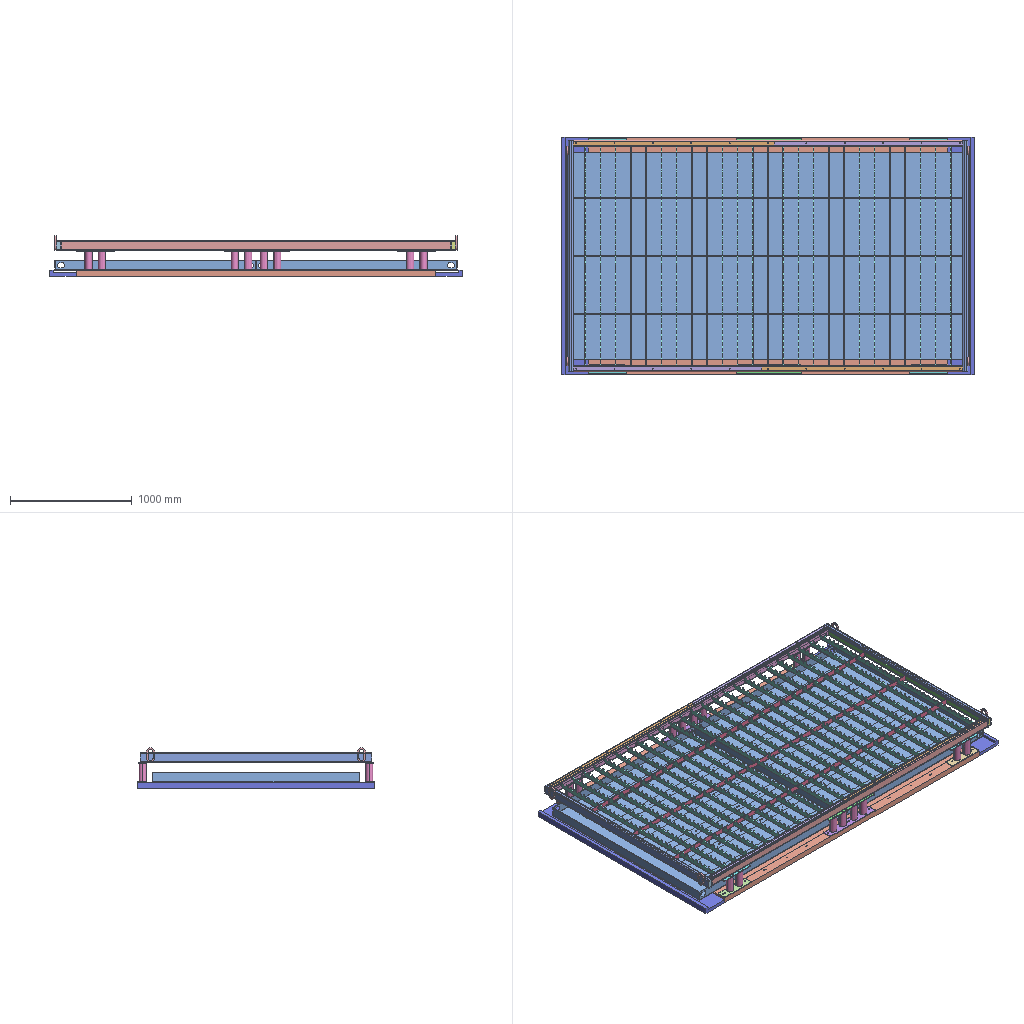Assembly | SolidWorks | 23 different items | 83 placed | box 3390 x 1950 x 331 mm
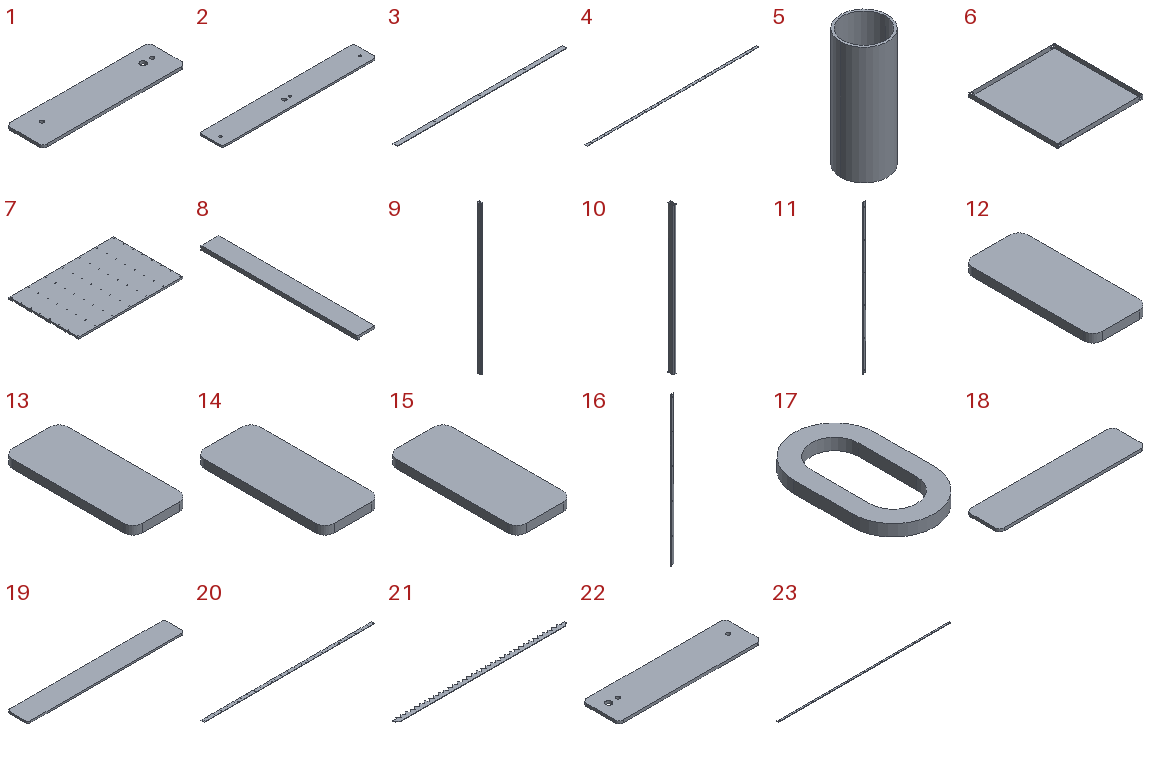Parts list (item | quantity | size | volume | features):
1 | x2 | 310 x 80 x 6 mm | 146885 mm3 | features FlatPattern 1, SMBaseFlange 1, SheetMetal 1
2 | x2 | 530 x 80 x 6 mm | 252184 mm3 | features FlatPattern 1, SMBaseFlange 1, SheetMetal 1
3 | x2 | 1790 x 45 x 4.5 mm | 360956 mm3 | features FlatPattern 1, SMBaseFlange 1, SheetMetal 1
4 | x3 | 3200 x 45 x 4.5 mm | 632235 mm3 | features Fillet 1, FlatPattern 1, SMBaseFlange 1, SheetMetal 1
5 | x16 | 60 x 60 x 150 mm | 80582 mm3 | features Extrusion 1
6 | x2 | 1650 x 1700 x 80 mm | 7628292 mm3 | features Extrusion 1, ICE 1, Shell 1
7 | x1 | 2950 x 1950 x 50 mm | 248660508 mm3 | features LPattern 4, ICE 2, FlatPattern 1, HoleWzd 1, SMBaseFlange 1, SheetMetal 1
8 | x2 | 220 x 1950 x 50 mm | 14040000 mm3 | features FlatPattern 1, ICE 1, SMBaseFlange 1, SheetMetal 1
9 | x2 | 40 x 80 x 3200 mm | 3306758 mm3 | features ICE 2, Extrusion 1, HoleWzd 1, LPattern 1
10 | x2 | 40 x 80 x 1900 mm | 1967677 mm3 | features Extrusion 1
11 | x2 | 40 x 19 x 1650 mm | 377391 mm3 | features FlatPattern 1, HoleWzd 1, LPattern 1, SMBaseFlange 1, SheetMetal 1
12 | x1 | 30 x 70 x 4.5 mm | 9353 mm3 | features FlatPattern 1, SMBaseFlange 1, SheetMetal 1
13 | x1 | 30 x 70 x 4.5 mm | 9353 mm3 | features FlatPattern 1, SMBaseFlange 1, SheetMetal 1
14 | x1 | 30 x 70 x 4.5 mm | 9353 mm3 | features FlatPattern 1, SMBaseFlange 1, SheetMetal 1
15 | x1 | 30 x 70 x 4.5 mm | 9353 mm3 | features FlatPattern 1, SMBaseFlange 1, SheetMetal 1
16 | x2 | 40 x 19 x 1550 mm | 354622 mm3 | features FlatPattern 1, HoleWzd 1, LPattern 1, SMBaseFlange 1, SheetMetal 1
17 | x4 | 70 x 120 x 10 mm | 40918 mm3 | features FlatPattern 1, SMBaseFlange 1, SheetMetal 1
18 | x4 | 310 x 70 x 6 mm | 129685 mm3 | features FlatPattern 1, SMBaseFlange 1, SheetMetal 1
19 | x2 | 530 x 70 x 6 mm | 222085 mm3 | features FlatPattern 1, SMBaseFlange 1, SheetMetal 1
20 | x2 | 3200 x 60 x 4.5 mm | 848029 mm3 | features FlatPattern 1, HoleWzd 1, ICE 1, SMBaseFlange 1, SheetMetal 1
21 | x25 | 1818 x 58.876 x 4.5 mm | 363940 mm3 | features Fillet 2, Chamfer 1, FlatPattern 1, SMBaseFlange 1, SheetMetal 1
22 | x2 | 310 x 80 x 6 mm | 146885 mm3 | features FlatPattern 1, SMBaseFlange 1, SheetMetal 1
23 | x2 | 3200 x 35 x 8 mm | 891006 mm3 | features FlatPattern 1, HoleWzd 1, SMBaseFlange 1, SheetMetal 1
Mates (type | each side: item.copy, entity, surface, feature):
Coincident | 9.1 face plane Boss-Extrude1 | 10.1 face plane Boss-Extrude1 | 3 times
Coincident | 10.1 face plane Boss-Extrude1 | 9.2 face plane Boss-Extrude1 | 3 times
Coincident | 9.2 face plane Boss-Extrude1 | 10.2 face plane Boss-Extrude1 | 3 times
Coincident | 9.1 face plane Boss-Extrude1 | 23.1 face plane Base-Flange1
Coincident | 10.1 face plane Boss-Extrude1 | 23.1 face plane Base-Flange1
DistanceDim | 9.1 face plane Boss-Extrude1 | 23.1 face plane Base-Flange1
Coincident | 9.2 face plane Boss-Extrude1 | 23.2 face plane Base-Flange1
Coincident | 10.2 face plane Boss-Extrude1 | 23.2 face plane Base-Flange1
Coincident | 23.1 face plane Base-Flange1 | 23.2 face plane Base-Flange1
Coincident | 23.1 face plane Base-Flange1 | 20.1 face plane Base-Flange1
Concentric | 23.1 face cylinder M10 Tapped Hole1 | 20.1 face cylinder M10 Tapped Hole1 | 2 times
Coincident | 23.2 face plane Base-Flange1 | 20.2 face plane Base-Flange1
Concentric | 23.2 face cylinder M10 Tapped Hole1 | 20.2 face cylinder M10 Tapped Hole1 | 2 times
Coincident | 23.2 face plane Base-Flange1 | 21.1 face plane Base-Flange1
DistanceDim | 21.1 face plane Base-Flange1 | 9.1 face plane Boss-Extrude1
Coincident | 20.2 face plane Cut-Extrude1 | 21.1 face plane Base-Flange1
Coincident | 9.1 face plane Boss-Extrude1 | 11.1 face plane Base-Flange1
Concentric | 9.1 face cylinder M8 Tapped Hole1 | 11.1 face cylinder M8 Tapped Hole1
Concentric | 9.1 face cylinder M8 Tapped Hole1 | 11.1 face cylinder LPattern1
Coincident | 9.1 face plane Boss-Extrude1 | 16.1 face plane Base-Flange1
Concentric | 9.1 face cylinder M8 Tapped Hole1 | 16.1 face cylinder M8 Tapped Hole1
Concentric | 9.1 face cylinder M8 Tapped Hole1 | 16.1 face cylinder LPattern1
Coincident | 9.2 face plane Boss-Extrude1 | 11.2 face plane Base-Flange1
Concentric | 9.2 face cylinder M8 Tapped Hole1 | 11.2 face cylinder M8 Tapped Hole1
Concentric | 9.2 face cylinder M8 Tapped Hole1 | 11.2 face cylinder LPattern1
Coincident | 9.2 face plane Boss-Extrude1 | 16.2 face plane Base-Flange1
Concentric | 9.2 face cylinder M8 Tapped Hole1 | 16.2 face cylinder M8 Tapped Hole1
Concentric | 9.2 face cylinder M8 Tapped Hole1 | 16.2 face cylinder LPattern1
Coincident | 10.1 face plane Boss-Extrude1 | 3.1 face plane Base-Flange1
Coincident | 23.2 face plane Base-Flange1 | 3.1 face plane Base-Flange1
DistanceDim | 20.2 face plane Base-Flange1 | 3.1 face plane Base-Flange1
InPlace | 4.1 plane | assembly plane
InPlace | 10.1 face plane Boss-Extrude1 | 12.1 plane
InPlace | 10.2 face plane Boss-Extrude1 | 13.1 plane
InPlace | 10.2 face plane Boss-Extrude1 | 14.1 plane
InPlace | 10.1 face plane Boss-Extrude1 | 15.1 plane
DistanceDim | 9.1 face plane Boss-Extrude1 | 7.1 face plane Base-Flange1 | 2 times
DistanceDim | 10.2 face plane Boss-Extrude1 | 7.1 face plane Base-Flange1
Coincident | 7.1 face plane Base-Flange1 | 8.1 face plane Base-Flange1 | 3 times
Coincident | 7.1 face plane Base-Flange1 | 8.2 face plane Base-Flange1 | 3 times
InPlace | 7.1 face plane Base-Flange1 | 22.1 plane
Coincident | 22.1 face plane Base-Flange1 | 5.1 face plane Boss-Extrude1
DistanceDim | 5.1 face cylinder Boss-Extrude1 | 9.2 face plane Boss-Extrude1
DistanceDim | 5.1 face cylinder Boss-Extrude1 | 22.1 face plane Base-Flange1
Parallel | 5.1 plane | assembly plane
InPlace | 5.2 face plane Boss-Extrude1 | 18.1 plane
Coincident | 7.1 face plane Base-Flange1 | 1.1 face plane Base-Flange1
Concentric | 7.1 face cylinder M8 Tapped Hole1 | 1.1 face cylinder Base-Flange1
Concentric | 7.1 face cylinder LPattern3 | 1.1 face cylinder Base-Flange1
InPlace | 7.1 face plane Base-Flange1 | 2.1 plane
InPlace | 5.3 face plane Boss-Extrude1 | 19.1 plane
Coincident | 10.2 face plane Boss-Extrude1 | 17.1 face plane Base-Flange1
DistanceDim | 17.1 face plane Base-Flange1 | 10.2 face plane Boss-Extrude1
DistanceDim | 17.1 face cylinder Base-Flange1 | 10.2 face plane Boss-Extrude1
Coincident | 7.1 face plane Base-Flange1 | 6.1 face plane Boss-Extrude1
DistanceDim | 6.1 face plane Boss-Extrude1 | 7.1 face plane Cut-Extrude1
DistanceDim | 8.1 face plane Base-Flange1 | 6.1 face plane Boss-Extrude1